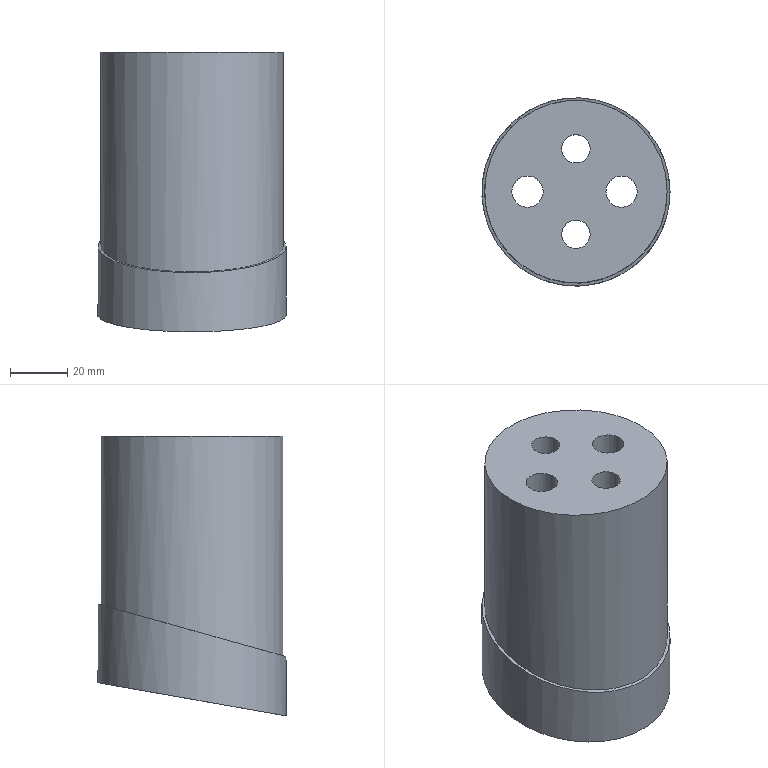Part | NX | features solid 2 | 1 solid | 17 faces | box 66 x 66 x 98.095 mm | volume 251323 mm3 | cylinder 10 | plane 5 | spline 2 | commonest cylinder face diameters 11 x4 10 x2 16 x2 64 x1 66 x1
STEP:
#1=CARTESIAN_POINT('',(502.403,-183.809,143.));
#2=VERTEX_POINT('',#1);
#3=CARTESIAN_POINT('',(496.903,-183.809,143.));
#4=DIRECTION('',(0.,0.,1.));
#5=DIRECTION('',(1.,0.,0.));
#6=AXIS2_PLACEMENT_3D('',#3,#4,#5);
#7=CIRCLE('',#6,5.5);
#8=EDGE_CURVE('',#2,#2,#7,.T.);
#9=ORIENTED_EDGE('',*,*,#8,.F.);
#10=EDGE_LOOP('',(#9));
#11=FACE_BOUND('',#10,.T.);
#12=CARTESIAN_POINT('',(469.403,-183.809,143.));
#13=VERTEX_POINT('',#12);
#14=CARTESIAN_POINT('',(463.903,-183.809,143.));
#15=DIRECTION('',(0.,0.,1.));
#16=DIRECTION('',(1.,0.,0.));
#17=AXIS2_PLACEMENT_3D('',#14,#15,#16);
#18=CIRCLE('',#17,5.5);
#19=EDGE_CURVE('',#13,#13,#18,.T.);
#20=ORIENTED_EDGE('',*,*,#19,.F.);
#21=EDGE_LOOP('',(#20));
#22=FACE_BOUND('',#21,.T.);
#23=CARTESIAN_POINT('',(485.903,-198.809,143.));
#24=VERTEX_POINT('',#23);
#25=CARTESIAN_POINT('',(480.903,-198.809,143.));
#26=DIRECTION('',(0.,0.,1.));
#27=DIRECTION('',(1.,0.,0.));
#28=AXIS2_PLACEMENT_3D('',#25,#26,#27);
#29=CIRCLE('',#28,5.);
#30=EDGE_CURVE('',#24,#24,#29,.T.);
#31=ORIENTED_EDGE('',*,*,#30,.F.);
#32=EDGE_LOOP('',(#31));
#33=FACE_BOUND('',#32,.T.);
#34=CARTESIAN_POINT('',(485.903,-168.809,143.));
#35=VERTEX_POINT('',#34);
#36=CARTESIAN_POINT('',(480.903,-168.809,143.));
#37=DIRECTION('',(0.,0.,1.));
#38=DIRECTION('',(1.,0.,0.));
#39=AXIS2_PLACEMENT_3D('',#36,#37,#38);
#40=CIRCLE('',#39,5.);
#41=EDGE_CURVE('',#35,#35,#40,.T.);
#42=ORIENTED_EDGE('',*,*,#41,.F.);
#43=EDGE_LOOP('',(#42));
#44=FACE_BOUND('',#43,.T.);
#45=CARTESIAN_POINT('',(512.903,-183.809,143.));
#46=VERTEX_POINT('',#45);
#47=CARTESIAN_POINT('',(480.903,-183.809,143.));
#48=DIRECTION('',(0.,0.,1.));
#49=DIRECTION('',(1.,0.,0.));
#50=AXIS2_PLACEMENT_3D('',#47,#48,#49);
#51=CIRCLE('',#50,32.);
#52=EDGE_CURVE('',#46,#46,#51,.T.);
#53=ORIENTED_EDGE('',*,*,#52,.T.);
#54=EDGE_LOOP('',(#53));
#55=FACE_BOUND('',#54,.T.);
#56=CARTESIAN_POINT('',(480.903,-183.809,143.));
#57=DIRECTION('',(0.,0.,1.));
#58=DIRECTION('',(1.,0.,0.));
#59=AXIS2_PLACEMENT_3D('',#56,#57,#58);
#60=PLANE('',#59);
#61=ADVANCED_FACE('',(#11,#22,#33,#44,#55),#60,.T.);
#62=CARTESIAN_POINT('',(486.398,-168.57,53.41));
#63=VERTEX_POINT('',#62);
#64=CARTESIAN_POINT('',(485.417,-172.905,52.646));
#65=CARTESIAN_POINT('',(486.981,-168.545,53.415));
#66=CARTESIAN_POINT('',(485.046,-164.339,54.156));
#67=CARTESIAN_POINT('',(480.639,-162.707,54.444));
#68=CARTESIAN_POINT('',(476.387,-164.715,54.09));
#69=CARTESIAN_POINT('',(474.827,-169.071,53.322));
#70=CARTESIAN_POINT('',(476.753,-173.273,52.581));
#71=CARTESIAN_POINT('',(481.163,-174.911,52.292));
#72=CARTESIAN_POINT('',(485.417,-172.905,52.646));
#73=CARTESIAN_POINT('',(486.981,-168.545,53.415));
#74=CARTESIAN_POINT('',(485.046,-164.339,54.156));
#75=B_SPLINE_CURVE_WITH_KNOTS('',3,(#64,#65,#66,#67,#68,#69,#70,#71,#72,#73,#74),.UNSPECIFIED.,.T.,.F.,(1,1,1,1,1,1,1,1,1,1,1,1,1,1,1),(-0.01299,-0.008662,-0.004331,0.,0.004331,0.008662,0.01299,0.01732,0.02165,0.02599,0.03032,0.03465,0.03898,0.04331,0.04764),.UNSPECIFIED.);
#76=EDGE_CURVE('',#63,#63,#75,.T.);
#77=ORIENTED_EDGE('',*,*,#76,.T.);
#78=EDGE_LOOP('',(#77));
#79=FACE_BOUND('',#78,.T.);
#80=CARTESIAN_POINT('',(471.571,-181.528,51.125));
#81=VERTEX_POINT('',#80);
#82=CARTESIAN_POINT('',(468.145,-176.009,52.098));
#83=CARTESIAN_POINT('',(472.391,-181.297,51.166));
#84=CARTESIAN_POINT('',(471.717,-187.972,49.989));
#85=CARTESIAN_POINT('',(466.488,-192.303,49.225));
#86=CARTESIAN_POINT('',(459.66,-191.607,49.348));
#87=CARTESIAN_POINT('',(455.417,-186.322,50.28));
#88=CARTESIAN_POINT('',(456.085,-179.656,51.455));
#89=CARTESIAN_POINT('',(461.311,-175.314,52.221));
#90=CARTESIAN_POINT('',(468.145,-176.009,52.098));
#91=CARTESIAN_POINT('',(472.391,-181.297,51.166));
#92=CARTESIAN_POINT('',(471.717,-187.972,49.989));
#93=B_SPLINE_CURVE_WITH_KNOTS('',3,(#82,#83,#84,#85,#86,#87,#88,#89,#90,#91,#92),.UNSPECIFIED.,.T.,.F.,(1,1,1,1,1,1,1,1,1,1,1,1,1,1,1),(-0.0189,-0.0126,-0.006299,0.,0.006299,0.0126,0.0189,0.0252,0.0315,0.0378,0.04409,0.05039,0.05669,0.06299,0.06929),.UNSPECIFIED.);
#94=EDGE_CURVE('',#81,#81,#93,.T.);
#95=ORIENTED_EDGE('',*,*,#94,.F.);
#96=EDGE_LOOP('',(#95));
#97=FACE_BOUND('',#96,.T.);
#98=CARTESIAN_POINT('',(504.571,-181.528,51.125));
#99=VERTEX_POINT('',#98);
#100=CARTESIAN_POINT('',(501.145,-176.009,52.098));
#101=CARTESIAN_POINT('',(505.391,-181.297,51.166));
#102=CARTESIAN_POINT('',(504.717,-187.972,49.989));
#103=CARTESIAN_POINT('',(499.488,-192.303,49.225));
#104=CARTESIAN_POINT('',(492.66,-191.607,49.348));
#105=CARTESIAN_POINT('',(488.417,-186.322,50.28));
#106=CARTESIAN_POINT('',(489.085,-179.656,51.455));
#107=CARTESIAN_POINT('',(494.311,-175.314,52.221));
#108=CARTESIAN_POINT('',(501.145,-176.009,52.098));
#109=CARTESIAN_POINT('',(505.391,-181.297,51.166));
#110=CARTESIAN_POINT('',(504.717,-187.972,49.989));
#111=B_SPLINE_CURVE_WITH_KNOTS('',3,(#100,#101,#102,#103,#104,#105,#106,#107,#108,#109,#110),.UNSPECIFIED.,.T.,.F.,(1,1,1,1,1,1,1,1,1,1,1,1,1,1,1),(-0.0189,-0.0126,-0.006299,0.,0.006299,0.0126,0.0189,0.0252,0.0315,0.0378,0.04409,0.05039,0.05669,0.06299,0.06929),.UNSPECIFIED.);
#112=EDGE_CURVE('',#99,#99,#111,.T.);
#113=ORIENTED_EDGE('',*,*,#112,.F.);
#114=EDGE_LOOP('',(#113));
#115=FACE_BOUND('',#114,.T.);
#116=CARTESIAN_POINT('',(448.176,-179.571,51.47));
#117=VERTEX_POINT('',#116);
#118=CARTESIAN_POINT('',(451.528,-166.978,53.691));
#119=CARTESIAN_POINT('',(447.331,-179.477,51.487));
#120=CARTESIAN_POINT('',(448.205,-192.541,49.183));
#121=CARTESIAN_POINT('',(453.984,-204.339,47.103));
#122=CARTESIAN_POINT('',(463.885,-213.086,45.561));
#123=CARTESIAN_POINT('',(476.456,-217.387,44.802));
#124=CARTESIAN_POINT('',(489.744,-216.507,44.958));
#125=CARTESIAN_POINT('',(501.641,-210.581,46.002));
#126=CARTESIAN_POINT('',(510.298,-200.599,47.763));
#127=CARTESIAN_POINT('',(514.466,-188.162,49.955));
#128=CARTESIAN_POINT('',(513.609,-175.102,52.258));
#129=CARTESIAN_POINT('',(507.844,-163.309,54.338));
#130=CARTESIAN_POINT('',(497.954,-154.549,55.882));
#131=CARTESIAN_POINT('',(485.376,-150.23,56.644));
#132=CARTESIAN_POINT('',(472.058,-151.109,56.489));
#133=CARTESIAN_POINT('',(460.17,-157.039,55.443));
#134=CARTESIAN_POINT('',(451.528,-166.978,53.691));
#135=CARTESIAN_POINT('',(447.331,-179.477,51.487));
#136=CARTESIAN_POINT('',(448.205,-192.541,49.183));
#137=B_SPLINE_CURVE_WITH_KNOTS('',3,(#118,#119,#120,#121,#122,#123,#124,#125,#126,#127,#128,#129,#130,#131,#132,#133,#134,#135,#136),.UNSPECIFIED.,.T.,.F.,(1,1,1,1,1,1,1,1,1,1,1,1,1,1,1,1,1,1,1,1,1,1,1),(-0.03898,-0.02598,-0.01299,0.,0.01299,0.02598,0.03898,0.05197,0.06496,0.07795,0.09095,0.1039,0.1169,0.1299,0.1429,0.1559,0.1689,0.1819,0.1949,0.2079,0.2209,0.2339,0.2469),.UNSPECIFIED.);
#138=EDGE_CURVE('',#117,#117,#137,.T.);
#139=ORIENTED_EDGE('',*,*,#138,.F.);
#140=EDGE_LOOP('',(#139));
#141=FACE_BOUND('',#140,.T.);
#142=CARTESIAN_POINT('',(486.395,-199.103,48.026));
#143=VERTEX_POINT('',#142);
#144=CARTESIAN_POINT('',(484.999,-203.327,47.282));
#145=CARTESIAN_POINT('',(486.978,-199.131,48.021));
#146=CARTESIAN_POINT('',(485.46,-194.765,48.791));
#147=CARTESIAN_POINT('',(481.242,-192.711,49.153));
#148=CARTESIAN_POINT('',(476.806,-194.292,48.875));
#149=CARTESIAN_POINT('',(474.83,-198.484,48.135));
#150=CARTESIAN_POINT('',(476.341,-202.846,47.366));
#151=CARTESIAN_POINT('',(480.56,-204.907,47.003));
#152=CARTESIAN_POINT('',(484.999,-203.327,47.282));
#153=CARTESIAN_POINT('',(486.978,-199.131,48.021));
#154=CARTESIAN_POINT('',(485.46,-194.765,48.791));
#155=B_SPLINE_CURVE_WITH_KNOTS('',3,(#144,#145,#146,#147,#148,#149,#150,#151,#152,#153,#154),.UNSPECIFIED.,.T.,.F.,(1,1,1,1,1,1,1,1,1,1,1,1,1,1,1),(-0.01299,-0.008662,-0.004331,0.,0.004331,0.008662,0.01299,0.01732,0.02165,0.02599,0.03032,0.03465,0.03898,0.04331,0.04764),.UNSPECIFIED.);
#156=EDGE_CURVE('',#143,#143,#155,.T.);
#157=ORIENTED_EDGE('',*,*,#156,.T.);
#158=EDGE_LOOP('',(#157));
#159=FACE_BOUND('',#158,.T.);
#160=CARTESIAN_POINT('',(514.51,-217.221,44.832));
#161=CARTESIAN_POINT('',(492.106,-217.221,44.832));
#162=CARTESIAN_POINT('',(469.701,-217.221,44.832));
#163=CARTESIAN_POINT('',(447.297,-217.221,44.832));
#164=CARTESIAN_POINT('',(514.51,-216.811,44.904));
#165=CARTESIAN_POINT('',(492.106,-216.811,44.904));
#166=CARTESIAN_POINT('',(469.701,-216.811,44.904));
#167=CARTESIAN_POINT('',(447.297,-216.811,44.904));
#168=CARTESIAN_POINT('',(514.51,-150.028,56.68));
#169=CARTESIAN_POINT('',(492.106,-150.028,56.68));
#170=CARTESIAN_POINT('',(469.701,-150.028,56.68));
#171=CARTESIAN_POINT('',(447.297,-150.028,56.68));
#172=B_SPLINE_SURFACE_WITH_KNOTS('',1,3,((#160,#161,#162,#163),(#164,#165,#166,#167),(#168,#169,#170,#171)),.PLANE_SURF.,.F.,.F.,.F.,(2,1,2),(4,4),(-0.005174,0.,0.8432),(0.05516,0.1224),.PIECEWISE_BEZIER_KNOTS.);
#173=ADVANCED_FACE('',(#79,#97,#115,#141,#159),#172,.F.);
#174=CARTESIAN_POINT('',(513.903,-183.809,74.898));
#175=VERTEX_POINT('',#174);
#176=CARTESIAN_POINT('',(512.237,-196.581,71.327));
#177=CARTESIAN_POINT('',(514.732,-183.795,74.902));
#178=CARTESIAN_POINT('',(512.252,-171.09,78.455));
#179=CARTESIAN_POINT('',(505.099,-160.127,81.521));
#180=CARTESIAN_POINT('',(494.13,-152.615,83.621));
#181=CARTESIAN_POINT('',(480.945,-149.914,84.377));
#182=CARTESIAN_POINT('',(467.743,-152.582,83.631));
#183=CARTESIAN_POINT('',(456.728,-160.099,81.529));
#184=CARTESIAN_POINT('',(449.555,-171.078,78.458));
#185=CARTESIAN_POINT('',(447.08,-183.793,74.903));
#186=CARTESIAN_POINT('',(449.543,-196.501,71.349));
#187=CARTESIAN_POINT('',(456.68,-207.461,68.284));
#188=CARTESIAN_POINT('',(467.637,-214.986,66.18));
#189=CARTESIAN_POINT('',(480.826,-217.707,65.419));
#190=CARTESIAN_POINT('',(494.068,-215.037,66.166));
#191=CARTESIAN_POINT('',(505.069,-207.519,68.268));
#192=CARTESIAN_POINT('',(512.237,-196.581,71.327));
#193=CARTESIAN_POINT('',(514.732,-183.795,74.902));
#194=CARTESIAN_POINT('',(512.252,-171.09,78.455));
#195=B_SPLINE_CURVE_WITH_KNOTS('',3,(#176,#177,#178,#179,#180,#181,#182,#183,#184,#185,#186,#187,#188,#189,#190,#191,#192,#193,#194),.UNSPECIFIED.,.T.,.F.,(1,1,1,1,1,1,1,1,1,1,1,1,1,1,1,1,1,1,1,1,1,1,1),(-0.03941,-0.02628,-0.01314,0.,0.01314,0.02628,0.03941,0.05255,0.06569,0.07883,0.09196,0.1051,0.1182,0.1314,0.1445,0.1577,0.1708,0.1839,0.1971,0.2102,0.2233,0.2365,0.2496),.UNSPECIFIED.);
#196=EDGE_CURVE('',#175,#175,#195,.T.);
#197=ORIENTED_EDGE('',*,*,#196,.F.);
#198=EDGE_LOOP('',(#197));
#199=FACE_BOUND('',#198,.T.);
#200=ORIENTED_EDGE('',*,*,#138,.T.);
#201=EDGE_LOOP('',(#200));
#202=FACE_BOUND('',#201,.T.);
#203=CARTESIAN_POINT('',(480.903,-183.809,-9.));
#204=DIRECTION('',(0.,0.,1.));
#205=DIRECTION('',(1.,0.,0.));
#206=AXIS2_PLACEMENT_3D('',#203,#204,#205);
#207=CYLINDRICAL_SURFACE('',#206,33.);
#208=ADVANCED_FACE('',(#199,#202),#207,.T.);
#209=CARTESIAN_POINT('',(502.403,-183.809,128.));
#210=VERTEX_POINT('',#209);
#211=CARTESIAN_POINT('',(496.903,-183.809,128.));
#212=DIRECTION('',(0.,0.,1.));
#213=DIRECTION('',(1.,0.,0.));
#214=AXIS2_PLACEMENT_3D('',#211,#212,#213);
#215=CIRCLE('',#214,5.5);
#216=EDGE_CURVE('',#210,#210,#215,.T.);
#217=ORIENTED_EDGE('',*,*,#216,.T.);
#218=EDGE_LOOP('',(#217));
#219=FACE_BOUND('',#218,.T.);
#220=CARTESIAN_POINT('',(504.903,-183.809,128.));
#221=VERTEX_POINT('',#220);
#222=CARTESIAN_POINT('',(496.903,-183.809,128.));
#223=DIRECTION('',(0.,0.,1.));
#224=DIRECTION('',(1.,0.,0.));
#225=AXIS2_PLACEMENT_3D('',#222,#223,#224);
#226=CIRCLE('',#225,8.);
#227=EDGE_CURVE('',#221,#221,#226,.F.);
#228=ORIENTED_EDGE('',*,*,#227,.T.);
#229=EDGE_LOOP('',(#228));
#230=FACE_BOUND('',#229,.T.);
#231=CARTESIAN_POINT('',(496.903,-183.809,128.));
#232=DIRECTION('',(0.,0.,1.));
#233=DIRECTION('',(-1.,0.,0.));
#234=AXIS2_PLACEMENT_3D('',#231,#232,#233);
#235=PLANE('',#234);
#236=ADVANCED_FACE('',(#219,#230),#235,.F.);
#237=ORIENTED_EDGE('',*,*,#112,.T.);
#238=EDGE_LOOP('',(#237));
#239=FACE_BOUND('',#238,.T.);
#240=ORIENTED_EDGE('',*,*,#227,.F.);
#241=EDGE_LOOP('',(#240));
#242=FACE_BOUND('',#241,.T.);
#243=CARTESIAN_POINT('',(496.903,-183.809,129.));
#244=DIRECTION('',(0.,0.,-1.));
#245=DIRECTION('',(1.,0.,0.));
#246=AXIS2_PLACEMENT_3D('',#243,#244,#245);
#247=CYLINDRICAL_SURFACE('',#246,8.);
#248=ADVANCED_FACE('',(#239,#242),#247,.F.);
#249=ORIENTED_EDGE('',*,*,#8,.T.);
#250=EDGE_LOOP('',(#249));
#251=FACE_BOUND('',#250,.T.);
#252=ORIENTED_EDGE('',*,*,#216,.F.);
#253=EDGE_LOOP('',(#252));
#254=FACE_BOUND('',#253,.T.);
#255=CARTESIAN_POINT('',(496.903,-183.809,128.));
#256=DIRECTION('',(0.,0.,1.));
#257=DIRECTION('',(-1.,0.,0.));
#258=AXIS2_PLACEMENT_3D('',#255,#256,#257);
#259=CYLINDRICAL_SURFACE('',#258,5.5);
#260=ADVANCED_FACE('',(#251,#254),#259,.F.);
#261=CARTESIAN_POINT('',(469.403,-183.809,128.));
#262=VERTEX_POINT('',#261);
#263=CARTESIAN_POINT('',(463.903,-183.809,128.));
#264=DIRECTION('',(0.,0.,1.));
#265=DIRECTION('',(1.,0.,0.));
#266=AXIS2_PLACEMENT_3D('',#263,#264,#265);
#267=CIRCLE('',#266,5.5);
#268=EDGE_CURVE('',#262,#262,#267,.T.);
#269=ORIENTED_EDGE('',*,*,#268,.T.);
#270=EDGE_LOOP('',(#269));
#271=FACE_BOUND('',#270,.T.);
#272=CARTESIAN_POINT('',(471.903,-183.809,128.));
#273=VERTEX_POINT('',#272);
#274=CARTESIAN_POINT('',(463.903,-183.809,128.));
#275=DIRECTION('',(0.,0.,1.));
#276=DIRECTION('',(1.,0.,0.));
#277=AXIS2_PLACEMENT_3D('',#274,#275,#276);
#278=CIRCLE('',#277,8.);
#279=EDGE_CURVE('',#273,#273,#278,.F.);
#280=ORIENTED_EDGE('',*,*,#279,.T.);
#281=EDGE_LOOP('',(#280));
#282=FACE_BOUND('',#281,.T.);
#283=CARTESIAN_POINT('',(463.903,-183.809,128.));
#284=DIRECTION('',(0.,0.,1.));
#285=DIRECTION('',(-1.,0.,0.));
#286=AXIS2_PLACEMENT_3D('',#283,#284,#285);
#287=PLANE('',#286);
#288=ADVANCED_FACE('',(#271,#282),#287,.F.);
#289=ORIENTED_EDGE('',*,*,#94,.T.);
#290=EDGE_LOOP('',(#289));
#291=FACE_BOUND('',#290,.T.);
#292=ORIENTED_EDGE('',*,*,#279,.F.);
#293=EDGE_LOOP('',(#292));
#294=FACE_BOUND('',#293,.T.);
#295=CARTESIAN_POINT('',(463.903,-183.809,129.));
#296=DIRECTION('',(0.,0.,-1.));
#297=DIRECTION('',(1.,0.,0.));
#298=AXIS2_PLACEMENT_3D('',#295,#296,#297);
#299=CYLINDRICAL_SURFACE('',#298,8.);
#300=ADVANCED_FACE('',(#291,#294),#299,.F.);
#301=ORIENTED_EDGE('',*,*,#19,.T.);
#302=EDGE_LOOP('',(#301));
#303=FACE_BOUND('',#302,.T.);
#304=ORIENTED_EDGE('',*,*,#268,.F.);
#305=EDGE_LOOP('',(#304));
#306=FACE_BOUND('',#305,.T.);
#307=CARTESIAN_POINT('',(463.903,-183.809,128.));
#308=DIRECTION('',(0.,0.,1.));
#309=DIRECTION('',(-1.,0.,0.));
#310=AXIS2_PLACEMENT_3D('',#307,#308,#309);
#311=CYLINDRICAL_SURFACE('',#310,5.5);
#312=ADVANCED_FACE('',(#303,#306),#311,.F.);
#313=CARTESIAN_POINT('',(475.903,-198.809,113.));
#314=VERTEX_POINT('',#313);
#315=CARTESIAN_POINT('',(480.903,-198.809,113.));
#316=DIRECTION('',(0.,0.,-1.));
#317=DIRECTION('',(-1.,0.,0.));
#318=AXIS2_PLACEMENT_3D('',#315,#316,#317);
#319=CIRCLE('',#318,5.);
#320=EDGE_CURVE('',#314,#314,#319,.T.);
#321=ORIENTED_EDGE('',*,*,#320,.T.);
#322=EDGE_LOOP('',(#321));
#323=FACE_BOUND('',#322,.T.);
#324=ORIENTED_EDGE('',*,*,#30,.T.);
#325=EDGE_LOOP('',(#324));
#326=FACE_BOUND('',#325,.T.);
#327=CARTESIAN_POINT('',(480.903,-198.809,133.));
#328=DIRECTION('',(0.,0.,1.));
#329=DIRECTION('',(-1.,0.,0.));
#330=AXIS2_PLACEMENT_3D('',#327,#328,#329);
#331=CYLINDRICAL_SURFACE('',#330,5.);
#332=ADVANCED_FACE('',(#323,#326),#331,.F.);
#333=CARTESIAN_POINT('',(475.903,-168.809,113.));
#334=VERTEX_POINT('',#333);
#335=CARTESIAN_POINT('',(480.903,-168.809,113.));
#336=DIRECTION('',(0.,0.,-1.));
#337=DIRECTION('',(-1.,0.,0.));
#338=AXIS2_PLACEMENT_3D('',#335,#336,#337);
#339=CIRCLE('',#338,5.);
#340=EDGE_CURVE('',#334,#334,#339,.T.);
#341=ORIENTED_EDGE('',*,*,#340,.T.);
#342=EDGE_LOOP('',(#341));
#343=FACE_BOUND('',#342,.T.);
#344=ORIENTED_EDGE('',*,*,#41,.T.);
#345=EDGE_LOOP('',(#344));
#346=FACE_BOUND('',#345,.T.);
#347=CARTESIAN_POINT('',(480.903,-168.809,133.));
#348=DIRECTION('',(0.,0.,1.));
#349=DIRECTION('',(-1.,0.,0.));
#350=AXIS2_PLACEMENT_3D('',#347,#348,#349);
#351=CYLINDRICAL_SURFACE('',#350,5.);
#352=ADVANCED_FACE('',(#343,#346),#351,.F.);
#353=CARTESIAN_POINT('',(475.403,-168.809,113.));
#354=VERTEX_POINT('',#353);
#355=CARTESIAN_POINT('',(480.903,-168.809,113.));
#356=DIRECTION('',(0.,0.,-1.));
#357=DIRECTION('',(-1.,0.,0.));
#358=AXIS2_PLACEMENT_3D('',#355,#356,#357);
#359=CIRCLE('',#358,5.5);
#360=EDGE_CURVE('',#354,#354,#359,.F.);
#361=ORIENTED_EDGE('',*,*,#360,.F.);
#362=EDGE_LOOP('',(#361));
#363=FACE_BOUND('',#362,.T.);
#364=ORIENTED_EDGE('',*,*,#340,.F.);
#365=EDGE_LOOP('',(#364));
#366=FACE_BOUND('',#365,.T.);
#367=CARTESIAN_POINT('',(480.903,-168.809,113.));
#368=DIRECTION('',(0.,0.,-1.));
#369=DIRECTION('',(-1.,0.,0.));
#370=AXIS2_PLACEMENT_3D('',#367,#368,#369);
#371=PLANE('',#370);
#372=ADVANCED_FACE('',(#363,#366),#371,.T.);
#373=ORIENTED_EDGE('',*,*,#76,.F.);
#374=EDGE_LOOP('',(#373));
#375=FACE_BOUND('',#374,.T.);
#376=ORIENTED_EDGE('',*,*,#360,.T.);
#377=EDGE_LOOP('',(#376));
#378=FACE_BOUND('',#377,.T.);
#379=CARTESIAN_POINT('',(480.903,-168.809,114.));
#380=DIRECTION('',(0.,0.,-1.));
#381=DIRECTION('',(-1.,0.,0.));
#382=AXIS2_PLACEMENT_3D('',#379,#380,#381);
#383=CYLINDRICAL_SURFACE('',#382,5.5);
#384=ADVANCED_FACE('',(#375,#378),#383,.F.);
#385=CARTESIAN_POINT('',(475.403,-198.809,113.));
#386=VERTEX_POINT('',#385);
#387=CARTESIAN_POINT('',(480.903,-198.809,113.));
#388=DIRECTION('',(0.,0.,-1.));
#389=DIRECTION('',(-1.,0.,0.));
#390=AXIS2_PLACEMENT_3D('',#387,#388,#389);
#391=CIRCLE('',#390,5.5);
#392=EDGE_CURVE('',#386,#386,#391,.F.);
#393=ORIENTED_EDGE('',*,*,#392,.F.);
#394=EDGE_LOOP('',(#393));
#395=FACE_BOUND('',#394,.T.);
#396=ORIENTED_EDGE('',*,*,#320,.F.);
#397=EDGE_LOOP('',(#396));
#398=FACE_BOUND('',#397,.T.);
#399=CARTESIAN_POINT('',(480.903,-198.809,113.));
#400=DIRECTION('',(0.,0.,-1.));
#401=DIRECTION('',(-1.,0.,0.));
#402=AXIS2_PLACEMENT_3D('',#399,#400,#401);
#403=PLANE('',#402);
#404=ADVANCED_FACE('',(#395,#398),#403,.T.);
#405=ORIENTED_EDGE('',*,*,#156,.F.);
#406=EDGE_LOOP('',(#405));
#407=FACE_BOUND('',#406,.T.);
#408=ORIENTED_EDGE('',*,*,#392,.T.);
#409=EDGE_LOOP('',(#408));
#410=FACE_BOUND('',#409,.T.);
#411=CARTESIAN_POINT('',(480.903,-198.809,114.));
#412=DIRECTION('',(0.,0.,-1.));
#413=DIRECTION('',(-1.,0.,0.));
#414=AXIS2_PLACEMENT_3D('',#411,#412,#413);
#415=CYLINDRICAL_SURFACE('',#414,5.5);
#416=ADVANCED_FACE('',(#407,#410),#415,.F.);
#417=ORIENTED_EDGE('',*,*,#196,.T.);
#418=EDGE_LOOP('',(#417));
#419=FACE_BOUND('',#418,.T.);
#420=CARTESIAN_POINT('',(505.776,-203.941,69.269));
#421=VERTEX_POINT('',#420);
#422=CARTESIAN_POINT('',(501.466,-208.599,67.966));
#423=CARTESIAN_POINT('',(507.444,-202.543,69.659));
#424=CARTESIAN_POINT('',(512.319,-193.234,72.263));
#425=CARTESIAN_POINT('',(513.56,-180.735,75.758));
#426=CARTESIAN_POINT('',(510.013,-168.672,79.131));
#427=CARTESIAN_POINT('',(502.081,-158.715,81.916));
#428=CARTESIAN_POINT('',(490.756,-152.46,83.665));
#429=CARTESIAN_POINT('',(477.753,-151.089,84.048));
#430=CARTESIAN_POINT('',(465.257,-154.917,82.978));
#431=CARTESIAN_POINT('',(455.378,-163.169,80.67));
#432=CARTESIAN_POINT('',(449.487,-174.369,77.538));
#433=CARTESIAN_POINT('',(448.246,-186.851,74.048));
#434=CARTESIAN_POINT('',(451.778,-198.918,70.673));
#435=CARTESIAN_POINT('',(459.702,-208.884,67.886));
#436=CARTESIAN_POINT('',(471.033,-215.155,66.133));
#437=CARTESIAN_POINT('',(484.068,-216.531,65.748));
#438=CARTESIAN_POINT('',(494.469,-213.329,66.644));
#439=CARTESIAN_POINT('',(501.466,-208.599,67.966));
#440=CARTESIAN_POINT('',(507.444,-202.543,69.659));
#441=CARTESIAN_POINT('',(512.319,-193.234,72.263));
#442=B_SPLINE_CURVE_WITH_KNOTS('',3,(#422,#423,#424,#425,#426,#427,#428,#429,#430,#431,#432,#433,#434,#435,#436,#437,#438,#439,#440,#441),.UNSPECIFIED.,.T.,.F.,(1,1,1,1,1,1,1,1,1,1,1,1,1,1,1,1,1,1,1,1,1,1,1,1),(-0.02548,-0.01274,-0.00637,0.,0.01274,0.02548,0.03822,0.05096,0.0637,0.07644,0.08918,0.1019,0.1147,0.1274,0.1401,0.1529,0.1656,0.1784,0.1911,0.1975,0.2038,0.2166,0.2293,0.2421),.UNSPECIFIED.);
#443=EDGE_CURVE('',#421,#421,#442,.T.);
#444=ORIENTED_EDGE('',*,*,#443,.F.);
#445=EDGE_LOOP('',(#444));
#446=FACE_BOUND('',#445,.T.);
#447=CARTESIAN_POINT('',(447.288,-217.337,65.523));
#448=CARTESIAN_POINT('',(469.625,-217.337,65.523));
#449=CARTESIAN_POINT('',(491.963,-217.337,65.523));
#450=CARTESIAN_POINT('',(514.3,-217.337,65.523));
#451=CARTESIAN_POINT('',(447.288,-194.97,71.777));
#452=CARTESIAN_POINT('',(469.625,-194.97,71.777));
#453=CARTESIAN_POINT('',(491.963,-194.97,71.777));
#454=CARTESIAN_POINT('',(514.3,-194.97,71.777));
#455=CARTESIAN_POINT('',(447.288,-172.604,78.032));
#456=CARTESIAN_POINT('',(469.625,-172.604,78.032));
#457=CARTESIAN_POINT('',(491.963,-172.604,78.032));
#458=CARTESIAN_POINT('',(514.3,-172.604,78.032));
#459=CARTESIAN_POINT('',(447.288,-150.237,84.286));
#460=CARTESIAN_POINT('',(469.625,-150.237,84.286));
#461=CARTESIAN_POINT('',(491.963,-150.237,84.286));
#462=CARTESIAN_POINT('',(514.3,-150.237,84.286));
#463=B_SPLINE_SURFACE_WITH_KNOTS('',3,3,((#447,#448,#449,#450),(#451,#452,#453,#454),(#455,#456,#457,#458),(#459,#460,#461,#462)),.UNSPECIFIED.,.F.,.F.,.F.,(4,4),(4,4),(0.2906,0.7328),(0.3672,0.7137),.UNSPECIFIED.);
#464=ADVANCED_FACE('',(#419,#446),#463,.F.);
#465=ORIENTED_EDGE('',*,*,#52,.F.);
#466=EDGE_LOOP('',(#465));
#467=FACE_BOUND('',#466,.T.);
#468=ORIENTED_EDGE('',*,*,#443,.T.);
#469=EDGE_LOOP('',(#468));
#470=FACE_BOUND('',#469,.T.);
#471=CARTESIAN_POINT('',(480.903,-183.809,114.));
#472=DIRECTION('',(0.,0.,1.));
#473=DIRECTION('',(1.,0.,0.));
#474=AXIS2_PLACEMENT_3D('',#471,#472,#473);
#475=CYLINDRICAL_SURFACE('',#474,32.);
#476=ADVANCED_FACE('',(#467,#470),#475,.T.);
#477=CLOSED_SHELL('',(#61,#173,#208,#236,#248,#260,#288,#300,#312,#332,#352,#372,#384,#404,#416,#464,#476));
#478=MANIFOLD_SOLID_BREP('',#477);
#479=(LENGTH_UNIT()NAMED_UNIT(*)SI_UNIT(.MILLI.,.METRE.));
#480=UNCERTAINTY_MEASURE_WITH_UNIT(LENGTH_MEASURE(0.0508),#479,'','');
#481=(NAMED_UNIT(*)PLANE_ANGLE_UNIT()SI_UNIT($,.RADIAN.));
#482=(NAMED_UNIT(*)SI_UNIT($,.STERADIAN.)SOLID_ANGLE_UNIT());
#483=(GEOMETRIC_REPRESENTATION_CONTEXT(3)GLOBAL_UNCERTAINTY_ASSIGNED_CONTEXT((#480))GLOBAL_UNIT_ASSIGNED_CONTEXT((#479,#481,#482))REPRESENTATION_CONTEXT('',''));
#484=ADVANCED_BREP_SHAPE_REPRESENTATION('',(#478),#483);